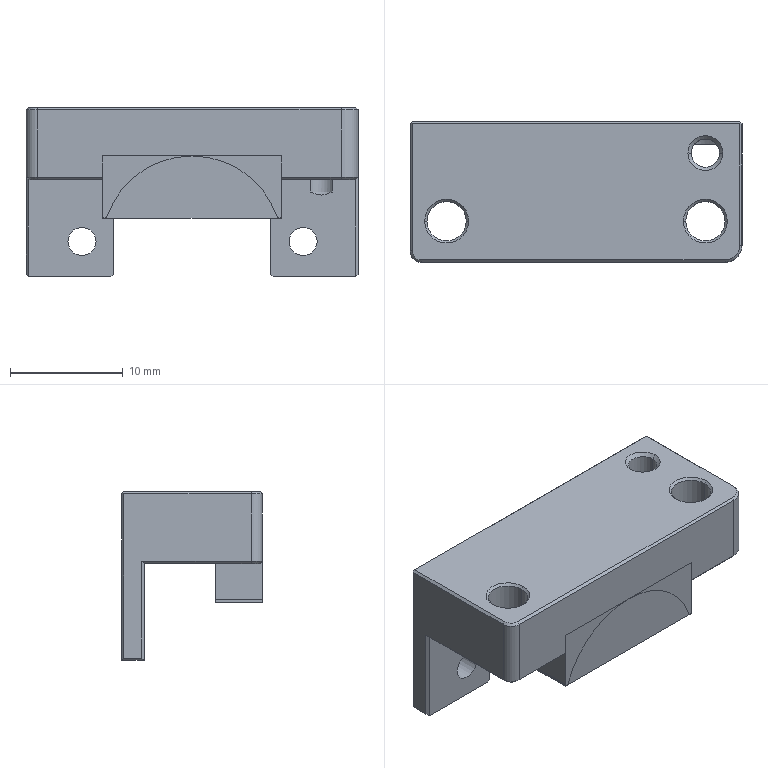NC program | NX | posted with a generic post | part box 29.5 x 12.5 x 15 mm
Whole program:
N10 G17 G21 G94 G90
(FLOOR_WALL_COPY , TOOL : D63)
N12 T03 M6
N14 G54
N16 G17 G0 G90 X-49.249 Y0. B0. C0. S6500 M3
N18 G43 Z30. H3
N20 Z3.
N22 G94 G1 Z0. F1250.
N24 X-46.249
N26 X46.249
N28 X49.249
N30 Z3.
N32 G0 Z30.
N34 M5
(DRILLING_COPY_1 , TOOL : D6A45)
N36 T01 M6
N38 G54
N40 G17 G0 G90 X11.5 Y-2.6 B0. C0. S5000 M3
N42 G43 Z30. H1
N44 G94 G81 G98 Z-1. F250. R3.
N46 X-11.5
N48 X11.5 Y3.45
N50 G80
N52 G0 X11.5 Y3.45 Z30.
N54 M5
(DRILLING_COPY_1_COPY , TOOL : 3.5ZT)
N56 T11 M6
N58 G54
N60 G17 G0 G90 X11.5 Y-2.6 B0. C0. S2000 M3
N62 G43 Z30. H11
N64 G94 G83 G98 Z-8.952 F250. Q2. R3.
N66 X-11.5
N68 G80
N70 G0 X-11.5 Y-2.6 Z30.
N72 M5
(DRILLING_COPY_1_COPY_COPY , TOOL : 2.5ZT)
N74 T12 M6
N76 G54
N78 G17 G0 G90 X11.5 Y3.45 B0. C0. S2546 M3
N80 G43 Z30. H12
N82 G94 G83 G98 Z-7.77 F150. Q2. R3.
N84 G80
N86 G0 X11.5 Y3.45 Z30.
N88 M5
(ADAPTIVE_MILLING_COPY , TOOL : D6JING)
N90 T16 M6
N92 G54
N94 G17 G0 G90 X-22.382 Y-0.025 B0. C0. S9500 M3
N96 G43 Z30. H16
N98 Z-14.
N100 G94 G1 Z-15. F1000.
N102 X-21.447 Y-0.373 F3000.
N104 G3 X-20.775 Y-0.025 R0.611
N106 X-20.402 Y2.706 R8.359
N108 G1 X-20.39 Y3.106
N110 X-20.38 Y3.556
N112 X-20.371 Y4.156
N114 X-20.364 Y4.956
N116 X-20.358 Y6.056
N118 X-20.355 Y7.756
N120 X-20.354 Y7.806
N122 X-20.35 Y7.906
N124 X-20.343 Y8.005
N126 X-20.332 Y8.105
N128 G2 X-17.896 Y10.999 R3.909
N130 X-13.443 Y11.789 R12.041
N132 X-6.244 Y11.845 R569.606
N134 G1 X16.256
N136 X16.356 Y11.843
N138 X16.456 Y11.838
N140 X16.506 Y11.833
N142 X16.605 Y11.822
N144 G2 X19.5 Y9.388 R3.907
N146 X20.273 Y5.285 R11.398
N148 X20.325 Y-8.064 R441.931
N150 X17.963 Y-10.956 R3.853
N152 X13.616 Y-11.761 R11.54
N154 X3.066 Y-11.831 R584.458
N156 G1 X-16.284 Y-11.844
N158 X-16.384 Y-11.841
N160 X-16.483 Y-11.834
N162 X-16.583 Y-11.824
N164 G2 X-19.489 Y-9.405 R3.886
N166 X-20.282 Y-5.055 R11.746
N168 X-20.092 Y1.435 R39.71
N170 G3 X-19.934 Y6.781 R593.208
N172 G2 X-16.929 Y10.491 R4.787
N174 X-12.437 Y11.353 R12.821
N176 X-3.888 Y11.44 R291.452
N178 G1 X14.762 Y11.441
N180 X14.862 Y11.439
N182 X14.962 Y11.436
N184 X15.012 Y11.433
N186 X15.112 Y11.426
N188 G2 X18.985 Y8.428 R4.734
N190 X19.864 Y3.687 R13.161
N192 X19.911 Y-6.761 R269.84
N194 X16.872 Y-10.496 R4.768
N196 X12.324 Y-11.339 R13.201
N198 X0.475 Y-11.428 R424.592
N200 X-15.274 Y-11.409 R822.076
N202 X-19.009 Y-8.368 R4.781
N204 X-19.86 Y-3.772 R13.19
N206 X-19.688 Y1.622 R50.718
N208 X-19.516 Y5.917 R85.746
N210 X-15.917 Y10.115 R5.468
N212 X-10.962 Y10.957 R15.234
N214 X2.387 Y11.037 R538.968
N216 G1 X13.437 Y11.036
N218 X13.637 Y11.034
N220 X13.787 Y11.029
N222 X13.937 Y11.022
N224 X14.086 Y11.011
N226 G2 X18.548 Y7.553 R5.342
N228 X19.45 Y2.611 R14.507
N230 X19.494 Y-5.737 R122.861
N232 X15.992 Y-10.057 R5.363
N234 X11.094 Y-10.931 R14.746
N236 X0.995 Y-11.024 R367.808
N238 X-14.154 Y-11.002 R840.579
N240 X-18.574 Y-7.488 R5.365
N242 X-19.414 Y-1.59 R14.731
N244 X-19.144 Y4.904 R231.582
N246 X-15.256 Y9.645 R5.9
N248 X-10.109 Y10.541 R15.886
N250 X-1.06 Y10.632 R334.893
N252 G1 X12.29
N254 X12.54 Y10.629
N256 X12.74 Y10.624
N258 X12.94 Y10.616
N260 X13.09 Y10.606
N262 G2 X18.125 Y6.767 R5.805
N264 X19.047 Y1.424 R16.011
N266 X19.076 Y-4.874 R71.369
N268 X15.265 Y-9.609 R5.807
N270 X10.121 Y-10.52 R15.734
N272 X1.122 Y-10.619 R323.136
N274 G1 X-12.328 Y-10.628
N276 X-12.528 Y-10.626
N278 X-12.728 Y-10.622
N280 X-12.928 Y-10.613
N282 X-13.078 Y-10.604
N284 G2 X-18.121 Y-6.776 R5.801
N286 X-18.951 Y-1.276 R14.133
N288 X-18.732 Y4.267 R63.859
N290 X-17.802 Y6.791 R8.055
N292 X-14.694 Y9.456 R3.739
N294 X-7.098 Y10.198 R33.598
N296 G1 X-6.298 Y10.208
N298 X-5.248 Y10.216
N300 X-3.998 Y10.222
N302 X-2.098 Y10.226
N304 X1.852 Y10.228
N306 X11.252
N308 G2 X15.177 Y9.317 R7.817
N310 X17.906 Y6.388 R3.589
N312 X18.691 Y-1.003 R32.047
N314 X18.56 Y-4.693 R18.335
N316 X16.204 Y-8.295 R5.835
N318 X13.579 Y-9.54 R6.096
N320 X7.576 Y-10.169 R26.327
N322 G1 X6.976 Y-10.181
N324 X6.276 Y-10.19
N326 X5.326 Y-10.199
N328 X4.076 Y-10.206
N330 X2.276 Y-10.212
N332 X-1.224 Y-10.216
N334 G2 X-12.373 Y-10.184 R399.692
N336 X-15.801 Y-8.805 R5.927
N338 G1 X-16.338 Y-8.49
N340 X-16.357 Y-8.476
N342 X-16.374 Y-8.461
N344 G2 X-17.288 Y-7.373 R4.977
N346 X-18.423 Y-2.945 R10.863
N348 X-18.319 Y3.646 R38.789
N350 X-17.9 Y5.284 R58.083
N352 X-17.799 Y6.814 R8.396
N354 G1 X-17.642 Y7.242
N356 X-17.453 Y7.658
N358 X-16.963 Y8.292
N360 X-16.543 Y8.665
N362 X-16.087 Y8.994
N364 X-15.709 Y9.153
N366 X-15.325 Y9.298
N368 G2 X-13.131 Y9.458 R23.437
N370 X-1.792 Y9.821 R119.553
N372 X11.507 Y9.786 R634.761
N374 X13.527 Y9.4 R11.882
N376 X15.215 Y9.312 R9.353
N378 G3 X15.303 Y10.627 R-0.66
N380 G1 X-14.127 Y10.72
N382 G3 X-14.788 Y10.061 R0.66
N384 X-14.13 Y9.4 R0.66
N386 G1 X13.57
N388 X14.57 Y9.397
N390 X14.988 Y9.345
N392 X15.403 Y9.277
N394 X15.783 Y9.122
N396 X16.157 Y8.953
N398 X16.792 Y8.463
N400 X17.165 Y8.043
N402 X17.494 Y7.587
N404 X17.653 Y7.209
N406 X17.798 Y6.825
N408 G2 X17.976 Y4.382 R30.677
N410 X18.237 Y-3.307 R53.05
N412 X17.872 Y-4.963 R9.577
N414 X16.188 Y-8.306 R4.472
N416 G3 X16.515 Y-9.381 R0.601
N418 G1 X16.784 Y-9.338 Z-14.977
N420 X17.039 Y-9.243 Z-14.955
N422 X17.652 Y-9.018 Z-14.9
N424 X18.605 Y-8.659
N426 G3 X18.888 Y-8.306 R0.627
N428 G1 X19.665 Y-5.674
N430 G3 X20.053 Y-3.215 R10.664
N432 G1 X20.234 Y4.317
N434 X20.186 Y4.485
N436 X20.095 Y4.634
N438 X19.418 Y5.428
N440 X19.144 Y5.758 Z-14.936
N442 X18.848 Y6.066 Z-14.972
N444 X18.696 Y6.144 Z-14.986
N446 X18.53 Y6.179 Z-15.
N448 G3 X17.9 Y5.58 R0.603
N450 G1 Y-4.73
N452 X17.897 Y-4.77
N454 X17.871 Y-4.969
N456 X17.808 Y-5.481
N458 X17.726 Y-5.991
N460 X17.499 Y-6.554
N462 X17.252 Y-7.108
N464 X16.887 Y-7.592
N466 X16.506 Y-8.063
N468 X16.028 Y-8.436
N470 X15.537 Y-8.793
N472 G2 X12.98 Y-9.417 R5.76
N474 X2.042 Y-9.806 R109.261
N476 X-11.557 Y-9.778 R536.43
N478 X-13.513 Y-9.387 R10.632
N480 X-15.32 Y-9.088 R5.749
N482 G1 X-15.838 Y-8.784
N484 G3 X-16.188 Y-10.013 R-0.66
N486 G1 X13.214 Y-10.72
N488 G3 X13.23 Y-9.4 R-0.66
N490 G1 X-13.52 Y-9.387
N492 G2 X-15.32 Y-9.088 R5.982
N494 G1 X-16.374 Y-8.461
N496 X-17.199 Y-7.552
N498 X-17.708 Y-6.486
N500 X-17.717 Y-6.464
N502 G2 X-18.04 Y-2.431 R28.225
N504 X-17.9 Y3.111 R33.299
N506 G1 Y5.311
N508 G3 X-18.561 Y5.97 R0.66
N510 X-19.22 Y5.311 R0.66
N512 G1 Y-5.177
N514 G3 X-18.559 Y-5.836 R0.66
N516 X-17.9 Y-5.177 R0.66
N518 G1 Y3.123
N520 G3 X-18.591 Y3.723 R0.608
N522 G1 X-19.363 Y3.614
N524 Z-12.
N526 G0 Z30.
(ZLEVEL_PROFILE_1_COPY , TOOL : D6JING)
N528 X-15.208 Y9.789
N530 Z-14.
N532 G1 Z-15. F1000.
N534 X-15.07 Y9.55
N536 G3 X-14.55 Y9.25 R0.6
N538 G1 X14.55
N540 G2 X16.671 Y8.371 R3.
N542 G1 X16.871 Y8.171
N544 G2 X17.75 Y6.05 R3.
N546 G1 Y-4.75
N548 G2 X13.25 Y-9.25 R4.5
N550 G1 X-13.747
N552 G2 X-14.016 Y-9.238 R3.
N554 G1 X-14.017 Y-9.241
N556 G2 X-17.75 Y-5.25 R4.
N558 G1 Y6.05
N560 G2 X-16.871 Y8.171 R3.
N562 G1 X-16.671 Y8.371
N564 G2 X-14.55 Y9.25 R3.
N566 G3 X-14.03 Y9.55 R0.6
N568 G1 X-13.857 Y9.85
N570 Z-14.
N572 G0 Z30.
N574 M5
(11_COPY_COPY , TOOL : D6A45)
N576 T01 M6
N578 G54
N580 G17 G0 G90 X12.45 Y-2.6 B0. C0. S9500 M3
N582 G43 Z30. H1
N584 Z3.
N586 G94 G1 Z-1. F1000.
N588 G3 X11.5 Y-1.65 R0.95
N590 X12.45 Y-2.6 R-0.95
N592 X12.15 Y-2.08 R0.6
N594 G1 Z2.
N596 G0 Z30.
N598 X-12.45 Y-2.6
N600 Z3.
N602 G1 Z-1.
N604 Y-2.601
N606 G3 X-11.499 Y-3.55 R0.95
N608 X-12.45 Y-2.6 R-0.95
N610 X-12.15 Y-3.12 R0.6
N612 G1 Z2.
N614 G0 Z30.
N616 X11.5 Y4.
N618 Z3.
N620 G1 Z-1.
N622 G3 X10.95 Y3.45 R0.55
N624 X11.5 Y4. R-0.55
N626 X11.24 Y3.85 R0.3
N628 G1 Z2.
N630 G0 Z30.
N632 X-15.565 Y8.039
N634 Z2.
N636 G1 Z-1.
N638 X-15.167 Y7.35
N640 G3 X-14.647 Y7.05 R0.6
N642 G1 X14.647
N644 G2 X15.549 Y6.153 R0.901
N646 G1 X15.55 Y5.859
N648 Y-4.767
N650 G2 X13.261 Y-7.05 R2.3
N652 G1 X-13.764
N654 G2 X-15.55 Y-5.25 R1.8
N656 G1 Y5.859
N658 X-15.549 Y6.153
N660 G2 X-14.647 Y7.05 R0.901
N662 G3 X-14.128 Y7.35 R0.6
N664 G1 X-13.608 Y8.25
N666 Z2.
N668 G0 Z30.
N670 M5
N672 M2